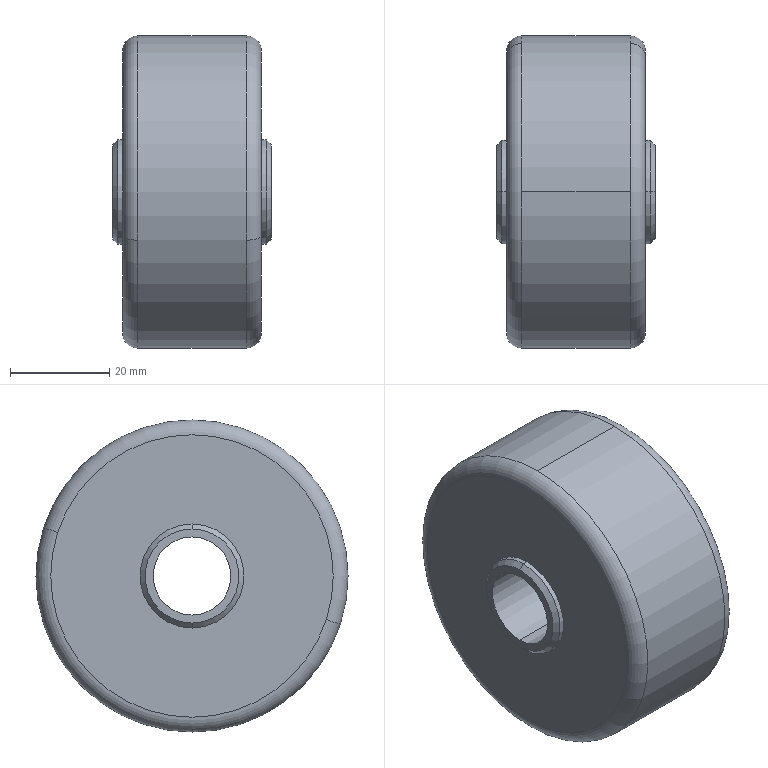Part | NX | features BREP 1 | 1 solid | 20 faces | box 32 x 63 x 63 mm | volume 81622 mm3 | cylinder 8 | cone 4 | plane 4 | torus 4 | commonest cylinder face diameters 21 x4 15.75 x2 63 x2
STEP:
#1=CARTESIAN_POINT('',(-16.,0.,-9.5));
#2=VERTEX_POINT('',#1);
#3=CARTESIAN_POINT('',(-16.,0.,9.5));
#4=VERTEX_POINT('',#3);
#5=CARTESIAN_POINT('',(-16.,0.,0.));
#6=DIRECTION('',(-1.,0.,0.));
#7=DIRECTION('',(0.,0.,-1.));
#8=AXIS2_PLACEMENT_3D('',#5,#6,#7);
#9=CIRCLE('',#8,9.5);
#10=EDGE_CURVE('',#2,#4,#9,.T.);
#11=ORIENTED_EDGE('',*,*,#10,.F.);
#12=CARTESIAN_POINT('',(-15.,0.,-10.5));
#13=VERTEX_POINT('',#12);
#14=CARTESIAN_POINT('',(-15.,0.,-10.5));
#15=DIRECTION('',(-0.7071,0.,0.7071));
#16=VECTOR('',#15,1000.);
#17=LINE('',#14,#16);
#18=EDGE_CURVE('',#2,#13,#17,.F.);
#19=ORIENTED_EDGE('',*,*,#18,.T.);
#20=CARTESIAN_POINT('',(-15.,0.,10.5));
#21=VERTEX_POINT('',#20);
#22=CARTESIAN_POINT('',(-15.,0.,0.));
#23=DIRECTION('',(-1.,0.,0.));
#24=DIRECTION('',(0.,0.,-1.));
#25=AXIS2_PLACEMENT_3D('',#22,#23,#24);
#26=CIRCLE('',#25,10.5);
#27=EDGE_CURVE('',#13,#21,#26,.T.);
#28=ORIENTED_EDGE('',*,*,#27,.T.);
#29=CARTESIAN_POINT('',(-15.,0.,10.5));
#30=DIRECTION('',(-0.7071,0.,-0.7071));
#31=VECTOR('',#30,1000.);
#32=LINE('',#29,#31);
#33=EDGE_CURVE('',#4,#21,#32,.F.);
#34=ORIENTED_EDGE('',*,*,#33,.F.);
#35=EDGE_LOOP('',(#11,#19,#28,#34));
#36=FACE_BOUND('',#35,.T.);
#37=CARTESIAN_POINT('',(-15.5,0.,0.));
#38=DIRECTION('',(1.,0.,0.));
#39=DIRECTION('',(0.,0.,1.));
#40=AXIS2_PLACEMENT_3D('',#37,#38,#39);
#41=CONICAL_SURFACE('',#40,10.,0.7854);
#42=ADVANCED_FACE('',(#36),#41,.T.);
#43=CARTESIAN_POINT('',(-15.,0.,0.));
#44=DIRECTION('',(-1.,0.,0.));
#45=DIRECTION('',(0.,0.,1.));
#46=AXIS2_PLACEMENT_3D('',#43,#44,#45);
#47=CIRCLE('',#46,10.5);
#48=EDGE_CURVE('',#21,#13,#47,.T.);
#49=ORIENTED_EDGE('',*,*,#48,.T.);
#50=ORIENTED_EDGE('',*,*,#18,.F.);
#51=CARTESIAN_POINT('',(-16.,0.,0.));
#52=DIRECTION('',(-1.,0.,0.));
#53=DIRECTION('',(0.,0.,1.));
#54=AXIS2_PLACEMENT_3D('',#51,#52,#53);
#55=CIRCLE('',#54,9.5);
#56=EDGE_CURVE('',#4,#2,#55,.T.);
#57=ORIENTED_EDGE('',*,*,#56,.F.);
#58=ORIENTED_EDGE('',*,*,#33,.T.);
#59=EDGE_LOOP('',(#49,#50,#57,#58));
#60=FACE_BOUND('',#59,.T.);
#61=CARTESIAN_POINT('',(-15.5,0.,0.));
#62=DIRECTION('',(1.,0.,0.));
#63=DIRECTION('',(0.,0.,-1.));
#64=AXIS2_PLACEMENT_3D('',#61,#62,#63);
#65=CONICAL_SURFACE('',#64,10.,0.7854);
#66=ADVANCED_FACE('',(#60),#65,.T.);
#67=ORIENTED_EDGE('',*,*,#56,.T.);
#68=ORIENTED_EDGE('',*,*,#10,.T.);
#69=EDGE_LOOP('',(#67,#68));
#70=FACE_BOUND('',#69,.T.);
#71=CARTESIAN_POINT('',(-16.,0.,7.875));
#72=VERTEX_POINT('',#71);
#73=CARTESIAN_POINT('',(-16.,0.,-7.875));
#74=VERTEX_POINT('',#73);
#75=CARTESIAN_POINT('',(-16.,0.,0.));
#76=DIRECTION('',(1.,0.,0.));
#77=DIRECTION('',(0.,0.,1.));
#78=AXIS2_PLACEMENT_3D('',#75,#76,#77);
#79=CIRCLE('',#78,7.875);
#80=EDGE_CURVE('',#72,#74,#79,.T.);
#81=ORIENTED_EDGE('',*,*,#80,.T.);
#82=CARTESIAN_POINT('',(-16.,0.,0.));
#83=DIRECTION('',(1.,0.,0.));
#84=DIRECTION('',(0.,0.,-1.));
#85=AXIS2_PLACEMENT_3D('',#82,#83,#84);
#86=CIRCLE('',#85,7.875);
#87=EDGE_CURVE('',#74,#72,#86,.T.);
#88=ORIENTED_EDGE('',*,*,#87,.T.);
#89=EDGE_LOOP('',(#81,#88));
#90=FACE_BOUND('',#89,.T.);
#91=CARTESIAN_POINT('',(-16.,9.5,0.));
#92=DIRECTION('',(-1.,0.,0.));
#93=DIRECTION('',(0.,0.,1.));
#94=AXIS2_PLACEMENT_3D('',#91,#92,#93);
#95=PLANE('',#94);
#96=ADVANCED_FACE('',(#70,#90),#95,.T.);
#97=ORIENTED_EDGE('',*,*,#87,.F.);
#98=CARTESIAN_POINT('',(16.,0.,-7.875));
#99=VERTEX_POINT('',#98);
#100=CARTESIAN_POINT('',(16.,0.,-7.875));
#101=DIRECTION('',(-1.,0.,0.));
#102=VECTOR('',#101,1000.);
#103=LINE('',#100,#102);
#104=EDGE_CURVE('',#74,#99,#103,.F.);
#105=ORIENTED_EDGE('',*,*,#104,.T.);
#106=CARTESIAN_POINT('',(16.,0.,7.875));
#107=VERTEX_POINT('',#106);
#108=CARTESIAN_POINT('',(16.,0.,0.));
#109=DIRECTION('',(-1.,0.,0.));
#110=DIRECTION('',(0.,0.,1.));
#111=AXIS2_PLACEMENT_3D('',#108,#109,#110);
#112=CIRCLE('',#111,7.875);
#113=EDGE_CURVE('',#107,#99,#112,.T.);
#114=ORIENTED_EDGE('',*,*,#113,.F.);
#115=CARTESIAN_POINT('',(16.,0.,7.875));
#116=DIRECTION('',(-1.,0.,0.));
#117=VECTOR('',#116,1000.);
#118=LINE('',#115,#117);
#119=EDGE_CURVE('',#72,#107,#118,.F.);
#120=ORIENTED_EDGE('',*,*,#119,.F.);
#121=EDGE_LOOP('',(#97,#105,#114,#120));
#122=FACE_BOUND('',#121,.T.);
#123=CARTESIAN_POINT('',(50.,0.,0.));
#124=DIRECTION('',(1.,0.,0.));
#125=DIRECTION('',(0.,0.,-1.));
#126=AXIS2_PLACEMENT_3D('',#123,#124,#125);
#127=CYLINDRICAL_SURFACE('',#126,7.875);
#128=ADVANCED_FACE('',(#122),#127,.F.);
#129=CARTESIAN_POINT('',(16.,0.,0.));
#130=DIRECTION('',(-1.,0.,0.));
#131=DIRECTION('',(0.,0.,-1.));
#132=AXIS2_PLACEMENT_3D('',#129,#130,#131);
#133=CIRCLE('',#132,7.875);
#134=EDGE_CURVE('',#99,#107,#133,.T.);
#135=ORIENTED_EDGE('',*,*,#134,.F.);
#136=ORIENTED_EDGE('',*,*,#104,.F.);
#137=ORIENTED_EDGE('',*,*,#80,.F.);
#138=ORIENTED_EDGE('',*,*,#119,.T.);
#139=EDGE_LOOP('',(#135,#136,#137,#138));
#140=FACE_BOUND('',#139,.T.);
#141=CARTESIAN_POINT('',(50.,0.,0.));
#142=DIRECTION('',(1.,0.,0.));
#143=DIRECTION('',(0.,0.,1.));
#144=AXIS2_PLACEMENT_3D('',#141,#142,#143);
#145=CYLINDRICAL_SURFACE('',#144,7.875);
#146=ADVANCED_FACE('',(#140),#145,.F.);
#147=CARTESIAN_POINT('',(16.,0.,9.5));
#148=VERTEX_POINT('',#147);
#149=CARTESIAN_POINT('',(16.,0.,-9.5));
#150=VERTEX_POINT('',#149);
#151=CARTESIAN_POINT('',(16.,0.,0.));
#152=DIRECTION('',(1.,0.,0.));
#153=DIRECTION('',(0.,0.,1.));
#154=AXIS2_PLACEMENT_3D('',#151,#152,#153);
#155=CIRCLE('',#154,9.5);
#156=EDGE_CURVE('',#148,#150,#155,.T.);
#157=ORIENTED_EDGE('',*,*,#156,.T.);
#158=CARTESIAN_POINT('',(16.,0.,0.));
#159=DIRECTION('',(1.,0.,0.));
#160=DIRECTION('',(0.,0.,-1.));
#161=AXIS2_PLACEMENT_3D('',#158,#159,#160);
#162=CIRCLE('',#161,9.5);
#163=EDGE_CURVE('',#150,#148,#162,.T.);
#164=ORIENTED_EDGE('',*,*,#163,.T.);
#165=EDGE_LOOP('',(#157,#164));
#166=FACE_BOUND('',#165,.T.);
#167=ORIENTED_EDGE('',*,*,#113,.T.);
#168=ORIENTED_EDGE('',*,*,#134,.T.);
#169=EDGE_LOOP('',(#167,#168));
#170=FACE_BOUND('',#169,.T.);
#171=CARTESIAN_POINT('',(16.,7.875,0.));
#172=DIRECTION('',(1.,0.,0.));
#173=DIRECTION('',(0.,1.,0.));
#174=AXIS2_PLACEMENT_3D('',#171,#172,#173);
#175=PLANE('',#174);
#176=ADVANCED_FACE('',(#166,#170),#175,.T.);
#177=CARTESIAN_POINT('',(15.,0.,-10.5));
#178=VERTEX_POINT('',#177);
#179=CARTESIAN_POINT('',(15.,0.,10.5));
#180=VERTEX_POINT('',#179);
#181=CARTESIAN_POINT('',(15.,0.,0.));
#182=DIRECTION('',(1.,0.,0.));
#183=DIRECTION('',(0.,0.,-1.));
#184=AXIS2_PLACEMENT_3D('',#181,#182,#183);
#185=CIRCLE('',#184,10.5);
#186=EDGE_CURVE('',#178,#180,#185,.T.);
#187=ORIENTED_EDGE('',*,*,#186,.T.);
#188=CARTESIAN_POINT('',(15.,0.,10.5));
#189=DIRECTION('',(0.7071,0.,-0.7071));
#190=VECTOR('',#189,1000.);
#191=LINE('',#188,#190);
#192=EDGE_CURVE('',#180,#148,#191,.T.);
#193=ORIENTED_EDGE('',*,*,#192,.T.);
#194=ORIENTED_EDGE('',*,*,#163,.F.);
#195=CARTESIAN_POINT('',(15.,0.,-10.5));
#196=DIRECTION('',(0.7071,0.,0.7071));
#197=VECTOR('',#196,1000.);
#198=LINE('',#195,#197);
#199=EDGE_CURVE('',#178,#150,#198,.T.);
#200=ORIENTED_EDGE('',*,*,#199,.F.);
#201=EDGE_LOOP('',(#187,#193,#194,#200));
#202=FACE_BOUND('',#201,.T.);
#203=CARTESIAN_POINT('',(15.5,0.,0.));
#204=DIRECTION('',(-1.,0.,0.));
#205=DIRECTION('',(0.,0.,1.));
#206=AXIS2_PLACEMENT_3D('',#203,#204,#205);
#207=CONICAL_SURFACE('',#206,10.,0.7854);
#208=ADVANCED_FACE('',(#202),#207,.T.);
#209=ORIENTED_EDGE('',*,*,#156,.F.);
#210=ORIENTED_EDGE('',*,*,#192,.F.);
#211=CARTESIAN_POINT('',(15.,0.,0.));
#212=DIRECTION('',(1.,0.,0.));
#213=DIRECTION('',(0.,0.,1.));
#214=AXIS2_PLACEMENT_3D('',#211,#212,#213);
#215=CIRCLE('',#214,10.5);
#216=EDGE_CURVE('',#180,#178,#215,.T.);
#217=ORIENTED_EDGE('',*,*,#216,.T.);
#218=ORIENTED_EDGE('',*,*,#199,.T.);
#219=EDGE_LOOP('',(#209,#210,#217,#218));
#220=FACE_BOUND('',#219,.T.);
#221=CARTESIAN_POINT('',(15.5,0.,0.));
#222=DIRECTION('',(-1.,0.,0.));
#223=DIRECTION('',(0.,0.,-1.));
#224=AXIS2_PLACEMENT_3D('',#221,#222,#223);
#225=CONICAL_SURFACE('',#224,10.,0.7854);
#226=ADVANCED_FACE('',(#220),#225,.T.);
#227=CARTESIAN_POINT('',(14.,0.,-10.5));
#228=VERTEX_POINT('',#227);
#229=CARTESIAN_POINT('',(14.,0.,10.5));
#230=VERTEX_POINT('',#229);
#231=CARTESIAN_POINT('',(14.,0.,0.));
#232=DIRECTION('',(-1.,0.,0.));
#233=DIRECTION('',(0.,0.,-1.));
#234=AXIS2_PLACEMENT_3D('',#231,#232,#233);
#235=CIRCLE('',#234,10.5);
#236=EDGE_CURVE('',#228,#230,#235,.T.);
#237=ORIENTED_EDGE('',*,*,#236,.F.);
#238=CARTESIAN_POINT('',(15.,0.,-10.5));
#239=DIRECTION('',(-1.,0.,0.));
#240=VECTOR('',#239,1000.);
#241=LINE('',#238,#240);
#242=EDGE_CURVE('',#228,#178,#241,.F.);
#243=ORIENTED_EDGE('',*,*,#242,.T.);
#244=ORIENTED_EDGE('',*,*,#216,.F.);
#245=CARTESIAN_POINT('',(15.,0.,10.5));
#246=DIRECTION('',(-1.,0.,0.));
#247=VECTOR('',#246,1000.);
#248=LINE('',#245,#247);
#249=EDGE_CURVE('',#230,#180,#248,.F.);
#250=ORIENTED_EDGE('',*,*,#249,.F.);
#251=EDGE_LOOP('',(#237,#243,#244,#250));
#252=FACE_BOUND('',#251,.T.);
#253=CARTESIAN_POINT('',(50.,0.,0.));
#254=DIRECTION('',(1.,0.,0.));
#255=DIRECTION('',(0.,0.,1.));
#256=AXIS2_PLACEMENT_3D('',#253,#254,#255);
#257=CYLINDRICAL_SURFACE('',#256,10.5);
#258=ADVANCED_FACE('',(#252),#257,.T.);
#259=ORIENTED_EDGE('',*,*,#186,.F.);
#260=ORIENTED_EDGE('',*,*,#242,.F.);
#261=CARTESIAN_POINT('',(14.,0.,0.));
#262=DIRECTION('',(-1.,0.,0.));
#263=DIRECTION('',(0.,0.,1.));
#264=AXIS2_PLACEMENT_3D('',#261,#262,#263);
#265=CIRCLE('',#264,10.5);
#266=EDGE_CURVE('',#230,#228,#265,.T.);
#267=ORIENTED_EDGE('',*,*,#266,.F.);
#268=ORIENTED_EDGE('',*,*,#249,.T.);
#269=EDGE_LOOP('',(#259,#260,#267,#268));
#270=FACE_BOUND('',#269,.T.);
#271=CARTESIAN_POINT('',(50.,0.,0.));
#272=DIRECTION('',(1.,0.,0.));
#273=DIRECTION('',(0.,0.,-1.));
#274=AXIS2_PLACEMENT_3D('',#271,#272,#273);
#275=CYLINDRICAL_SURFACE('',#274,10.5);
#276=ADVANCED_FACE('',(#270),#275,.T.);
#277=CARTESIAN_POINT('',(14.,27.105,8.807));
#278=VERTEX_POINT('',#277);
#279=CARTESIAN_POINT('',(14.,-27.105,-8.807));
#280=VERTEX_POINT('',#279);
#281=CARTESIAN_POINT('',(14.,0.,0.));
#282=DIRECTION('',(1.,0.,0.));
#283=DIRECTION('',(0.,0.9511,0.309));
#284=AXIS2_PLACEMENT_3D('',#281,#282,#283);
#285=CIRCLE('',#284,28.5);
#286=EDGE_CURVE('',#278,#280,#285,.T.);
#287=ORIENTED_EDGE('',*,*,#286,.T.);
#288=CARTESIAN_POINT('',(14.,0.,0.));
#289=DIRECTION('',(1.,0.,0.));
#290=DIRECTION('',(0.,-0.9511,-0.309));
#291=AXIS2_PLACEMENT_3D('',#288,#289,#290);
#292=CIRCLE('',#291,28.5);
#293=EDGE_CURVE('',#280,#278,#292,.T.);
#294=ORIENTED_EDGE('',*,*,#293,.T.);
#295=EDGE_LOOP('',(#287,#294));
#296=FACE_BOUND('',#295,.T.);
#297=ORIENTED_EDGE('',*,*,#266,.T.);
#298=ORIENTED_EDGE('',*,*,#236,.T.);
#299=EDGE_LOOP('',(#297,#298));
#300=FACE_BOUND('',#299,.T.);
#301=CARTESIAN_POINT('',(14.,10.5,0.));
#302=DIRECTION('',(1.,0.,0.));
#303=DIRECTION('',(0.,1.,0.));
#304=AXIS2_PLACEMENT_3D('',#301,#302,#303);
#305=PLANE('',#304);
#306=ADVANCED_FACE('',(#296,#300),#305,.T.);
#307=CARTESIAN_POINT('',(11.,-29.958,-9.734));
#308=VERTEX_POINT('',#307);
#309=CARTESIAN_POINT('',(11.,0.,-31.5));
#310=VERTEX_POINT('',#309);
#311=CARTESIAN_POINT('',(11.,0.,0.));
#312=DIRECTION('',(1.,0.,0.));
#313=DIRECTION('',(0.,-0.9511,-0.309));
#314=AXIS2_PLACEMENT_3D('',#311,#312,#313);
#315=CIRCLE('',#314,31.5);
#316=EDGE_CURVE('',#308,#310,#315,.T.);
#317=ORIENTED_EDGE('',*,*,#316,.T.);
#318=CARTESIAN_POINT('',(11.,29.958,9.734));
#319=VERTEX_POINT('',#318);
#320=CARTESIAN_POINT('',(11.,0.,0.));
#321=DIRECTION('',(1.,0.,0.));
#322=DIRECTION('',(0.,0.,-1.));
#323=AXIS2_PLACEMENT_3D('',#320,#321,#322);
#324=CIRCLE('',#323,31.5);
#325=EDGE_CURVE('',#310,#319,#324,.T.);
#326=ORIENTED_EDGE('',*,*,#325,.T.);
#327=CARTESIAN_POINT('',(11.,27.105,8.807));
#328=DIRECTION('',(0.,0.309,-0.9511));
#329=DIRECTION('',(0.,0.9511,0.309));
#330=AXIS2_PLACEMENT_3D('',#327,#328,#329);
#331=CIRCLE('',#330,3.);
#332=EDGE_CURVE('',#319,#278,#331,.T.);
#333=ORIENTED_EDGE('',*,*,#332,.T.);
#334=ORIENTED_EDGE('',*,*,#293,.F.);
#335=CARTESIAN_POINT('',(11.,-27.105,-8.807));
#336=DIRECTION('',(0.,-0.309,0.9511));
#337=DIRECTION('',(0.,-0.9511,-0.309));
#338=AXIS2_PLACEMENT_3D('',#335,#336,#337);
#339=CIRCLE('',#338,3.);
#340=EDGE_CURVE('',#308,#280,#339,.T.);
#341=ORIENTED_EDGE('',*,*,#340,.F.);
#342=EDGE_LOOP('',(#317,#326,#333,#334,#341));
#343=FACE_BOUND('',#342,.T.);
#344=CARTESIAN_POINT('',(11.,0.,0.));
#345=DIRECTION('',(1.,0.,0.));
#346=DIRECTION('',(0.,-0.9511,-0.309));
#347=AXIS2_PLACEMENT_3D('',#344,#345,#346);
#348=TOROIDAL_SURFACE('',#347,28.5,3.);
#349=ADVANCED_FACE('',(#343),#348,.T.);
#350=ORIENTED_EDGE('',*,*,#286,.F.);
#351=ORIENTED_EDGE('',*,*,#332,.F.);
#352=CARTESIAN_POINT('',(11.,0.,31.5));
#353=VERTEX_POINT('',#352);
#354=CARTESIAN_POINT('',(11.,0.,0.));
#355=DIRECTION('',(1.,0.,0.));
#356=DIRECTION('',(0.,0.9511,0.309));
#357=AXIS2_PLACEMENT_3D('',#354,#355,#356);
#358=CIRCLE('',#357,31.5);
#359=EDGE_CURVE('',#319,#353,#358,.T.);
#360=ORIENTED_EDGE('',*,*,#359,.T.);
#361=CARTESIAN_POINT('',(11.,0.,0.));
#362=DIRECTION('',(1.,0.,0.));
#363=DIRECTION('',(0.,0.,1.));
#364=AXIS2_PLACEMENT_3D('',#361,#362,#363);
#365=CIRCLE('',#364,31.5);
#366=EDGE_CURVE('',#353,#308,#365,.T.);
#367=ORIENTED_EDGE('',*,*,#366,.T.);
#368=ORIENTED_EDGE('',*,*,#340,.T.);
#369=EDGE_LOOP('',(#350,#351,#360,#367,#368));
#370=FACE_BOUND('',#369,.T.);
#371=CARTESIAN_POINT('',(11.,0.,0.));
#372=DIRECTION('',(1.,0.,0.));
#373=DIRECTION('',(0.,0.9511,0.309));
#374=AXIS2_PLACEMENT_3D('',#371,#372,#373);
#375=TOROIDAL_SURFACE('',#374,28.5,3.);
#376=ADVANCED_FACE('',(#370),#375,.T.);
#377=CARTESIAN_POINT('',(-11.,-29.958,-9.734));
#378=VERTEX_POINT('',#377);
#379=CARTESIAN_POINT('',(-11.,0.,31.5));
#380=VERTEX_POINT('',#379);
#381=CARTESIAN_POINT('',(-11.,0.,0.));
#382=DIRECTION('',(-1.,0.,0.));
#383=DIRECTION('',(0.,-0.9511,-0.309));
#384=AXIS2_PLACEMENT_3D('',#381,#382,#383);
#385=CIRCLE('',#384,31.5);
#386=EDGE_CURVE('',#378,#380,#385,.T.);
#387=ORIENTED_EDGE('',*,*,#386,.F.);
#388=CARTESIAN_POINT('',(-11.,0.,-31.5));
#389=VERTEX_POINT('',#388);
#390=CARTESIAN_POINT('',(-11.,0.,0.));
#391=DIRECTION('',(-1.,0.,0.));
#392=DIRECTION('',(0.,0.,-1.));
#393=AXIS2_PLACEMENT_3D('',#390,#391,#392);
#394=CIRCLE('',#393,31.5);
#395=EDGE_CURVE('',#389,#378,#394,.T.);
#396=ORIENTED_EDGE('',*,*,#395,.F.);
#397=CARTESIAN_POINT('',(11.,0.,-31.5));
#398=DIRECTION('',(-1.,0.,0.));
#399=VECTOR('',#398,1000.);
#400=LINE('',#397,#399);
#401=EDGE_CURVE('',#389,#310,#400,.F.);
#402=ORIENTED_EDGE('',*,*,#401,.T.);
#403=ORIENTED_EDGE('',*,*,#316,.F.);
#404=ORIENTED_EDGE('',*,*,#366,.F.);
#405=CARTESIAN_POINT('',(11.,0.,31.5));
#406=DIRECTION('',(-1.,0.,0.));
#407=VECTOR('',#406,1000.);
#408=LINE('',#405,#407);
#409=EDGE_CURVE('',#380,#353,#408,.F.);
#410=ORIENTED_EDGE('',*,*,#409,.F.);
#411=EDGE_LOOP('',(#387,#396,#402,#403,#404,#410));
#412=FACE_BOUND('',#411,.T.);
#413=CARTESIAN_POINT('',(50.,0.,0.));
#414=DIRECTION('',(1.,0.,0.));
#415=DIRECTION('',(0.,0.,1.));
#416=AXIS2_PLACEMENT_3D('',#413,#414,#415);
#417=CYLINDRICAL_SURFACE('',#416,31.5);
#418=ADVANCED_FACE('',(#412),#417,.T.);
#419=ORIENTED_EDGE('',*,*,#359,.F.);
#420=ORIENTED_EDGE('',*,*,#325,.F.);
#421=ORIENTED_EDGE('',*,*,#401,.F.);
#422=CARTESIAN_POINT('',(-11.,29.958,9.734));
#423=VERTEX_POINT('',#422);
#424=CARTESIAN_POINT('',(-11.,0.,0.));
#425=DIRECTION('',(-1.,0.,0.));
#426=DIRECTION('',(0.,0.9511,0.309));
#427=AXIS2_PLACEMENT_3D('',#424,#425,#426);
#428=CIRCLE('',#427,31.5);
#429=EDGE_CURVE('',#423,#389,#428,.T.);
#430=ORIENTED_EDGE('',*,*,#429,.F.);
#431=CARTESIAN_POINT('',(-11.,0.,0.));
#432=DIRECTION('',(-1.,0.,0.));
#433=DIRECTION('',(0.,0.,1.));
#434=AXIS2_PLACEMENT_3D('',#431,#432,#433);
#435=CIRCLE('',#434,31.5);
#436=EDGE_CURVE('',#380,#423,#435,.T.);
#437=ORIENTED_EDGE('',*,*,#436,.F.);
#438=ORIENTED_EDGE('',*,*,#409,.T.);
#439=EDGE_LOOP('',(#419,#420,#421,#430,#437,#438));
#440=FACE_BOUND('',#439,.T.);
#441=CARTESIAN_POINT('',(50.,0.,0.));
#442=DIRECTION('',(1.,0.,0.));
#443=DIRECTION('',(0.,0.,-1.));
#444=AXIS2_PLACEMENT_3D('',#441,#442,#443);
#445=CYLINDRICAL_SURFACE('',#444,31.5);
#446=ADVANCED_FACE('',(#440),#445,.T.);
#447=ORIENTED_EDGE('',*,*,#386,.T.);
#448=ORIENTED_EDGE('',*,*,#436,.T.);
#449=CARTESIAN_POINT('',(-14.,27.105,8.807));
#450=VERTEX_POINT('',#449);
#451=CARTESIAN_POINT('',(-11.,27.105,8.807));
#452=DIRECTION('',(0.,0.309,-0.9511));
#453=DIRECTION('',(-1.,0.,0.));
#454=AXIS2_PLACEMENT_3D('',#451,#452,#453);
#455=CIRCLE('',#454,3.);
#456=EDGE_CURVE('',#450,#423,#455,.T.);
#457=ORIENTED_EDGE('',*,*,#456,.F.);
#458=CARTESIAN_POINT('',(-14.,-27.105,-8.807));
#459=VERTEX_POINT('',#458);
#460=CARTESIAN_POINT('',(-14.,0.,0.));
#461=DIRECTION('',(-1.,0.,0.));
#462=DIRECTION('',(0.,-0.9511,-0.309));
#463=AXIS2_PLACEMENT_3D('',#460,#461,#462);
#464=CIRCLE('',#463,28.5);
#465=EDGE_CURVE('',#459,#450,#464,.T.);
#466=ORIENTED_EDGE('',*,*,#465,.F.);
#467=CARTESIAN_POINT('',(-11.,-27.105,-8.807));
#468=DIRECTION('',(0.,-0.309,0.9511));
#469=DIRECTION('',(-1.,0.,0.));
#470=AXIS2_PLACEMENT_3D('',#467,#468,#469);
#471=CIRCLE('',#470,3.);
#472=EDGE_CURVE('',#459,#378,#471,.T.);
#473=ORIENTED_EDGE('',*,*,#472,.T.);
#474=EDGE_LOOP('',(#447,#448,#457,#466,#473));
#475=FACE_BOUND('',#474,.T.);
#476=CARTESIAN_POINT('',(-11.,0.,0.));
#477=DIRECTION('',(1.,0.,0.));
#478=DIRECTION('',(0.,0.9511,0.309));
#479=AXIS2_PLACEMENT_3D('',#476,#477,#478);
#480=TOROIDAL_SURFACE('',#479,28.5,3.);
#481=ADVANCED_FACE('',(#475),#480,.T.);
#482=CARTESIAN_POINT('',(-14.,0.,0.));
#483=DIRECTION('',(-1.,0.,0.));
#484=DIRECTION('',(0.,0.,-1.));
#485=AXIS2_PLACEMENT_3D('',#482,#483,#484);
#486=CIRCLE('',#485,28.5);
#487=EDGE_CURVE('',#450,#459,#486,.T.);
#488=ORIENTED_EDGE('',*,*,#487,.F.);
#489=ORIENTED_EDGE('',*,*,#456,.T.);
#490=ORIENTED_EDGE('',*,*,#429,.T.);
#491=ORIENTED_EDGE('',*,*,#395,.T.);
#492=ORIENTED_EDGE('',*,*,#472,.F.);
#493=EDGE_LOOP('',(#488,#489,#490,#491,#492));
#494=FACE_BOUND('',#493,.T.);
#495=CARTESIAN_POINT('',(-11.,0.,0.));
#496=DIRECTION('',(1.,0.,0.));
#497=DIRECTION('',(0.,-0.9511,-0.309));
#498=AXIS2_PLACEMENT_3D('',#495,#496,#497);
#499=TOROIDAL_SURFACE('',#498,28.5,3.);
#500=ADVANCED_FACE('',(#494),#499,.T.);
#501=ORIENTED_EDGE('',*,*,#465,.T.);
#502=ORIENTED_EDGE('',*,*,#487,.T.);
#503=EDGE_LOOP('',(#501,#502));
#504=FACE_BOUND('',#503,.T.);
#505=CARTESIAN_POINT('',(-14.,0.,10.5));
#506=VERTEX_POINT('',#505);
#507=CARTESIAN_POINT('',(-14.,0.,-10.5));
#508=VERTEX_POINT('',#507);
#509=CARTESIAN_POINT('',(-14.,0.,0.));
#510=DIRECTION('',(1.,0.,0.));
#511=DIRECTION('',(0.,0.,1.));
#512=AXIS2_PLACEMENT_3D('',#509,#510,#511);
#513=CIRCLE('',#512,10.5);
#514=EDGE_CURVE('',#506,#508,#513,.T.);
#515=ORIENTED_EDGE('',*,*,#514,.T.);
#516=CARTESIAN_POINT('',(-14.,0.,0.));
#517=DIRECTION('',(1.,0.,0.));
#518=DIRECTION('',(0.,0.,-1.));
#519=AXIS2_PLACEMENT_3D('',#516,#517,#518);
#520=CIRCLE('',#519,10.5);
#521=EDGE_CURVE('',#508,#506,#520,.T.);
#522=ORIENTED_EDGE('',*,*,#521,.T.);
#523=EDGE_LOOP('',(#515,#522));
#524=FACE_BOUND('',#523,.T.);
#525=CARTESIAN_POINT('',(-14.,28.5,0.));
#526=DIRECTION('',(-1.,0.,0.));
#527=DIRECTION('',(0.,0.,1.));
#528=AXIS2_PLACEMENT_3D('',#525,#526,#527);
#529=PLANE('',#528);
#530=ADVANCED_FACE('',(#504,#524),#529,.T.);
#531=ORIENTED_EDGE('',*,*,#521,.F.);
#532=CARTESIAN_POINT('',(-14.,0.,-10.5));
#533=DIRECTION('',(-1.,0.,0.));
#534=VECTOR('',#533,1000.);
#535=LINE('',#532,#534);
#536=EDGE_CURVE('',#13,#508,#535,.F.);
#537=ORIENTED_EDGE('',*,*,#536,.F.);
#538=ORIENTED_EDGE('',*,*,#48,.F.);
#539=CARTESIAN_POINT('',(-14.,0.,10.5));
#540=DIRECTION('',(-1.,0.,0.));
#541=VECTOR('',#540,1000.);
#542=LINE('',#539,#541);
#543=EDGE_CURVE('',#21,#506,#542,.F.);
#544=ORIENTED_EDGE('',*,*,#543,.T.);
#545=EDGE_LOOP('',(#531,#537,#538,#544));
#546=FACE_BOUND('',#545,.T.);
#547=CARTESIAN_POINT('',(50.,0.,0.));
#548=DIRECTION('',(1.,0.,0.));
#549=DIRECTION('',(0.,0.,-1.));
#550=AXIS2_PLACEMENT_3D('',#547,#548,#549);
#551=CYLINDRICAL_SURFACE('',#550,10.5);
#552=ADVANCED_FACE('',(#546),#551,.T.);
#553=ORIENTED_EDGE('',*,*,#27,.F.);
#554=ORIENTED_EDGE('',*,*,#536,.T.);
#555=ORIENTED_EDGE('',*,*,#514,.F.);
#556=ORIENTED_EDGE('',*,*,#543,.F.);
#557=EDGE_LOOP('',(#553,#554,#555,#556));
#558=FACE_BOUND('',#557,.T.);
#559=CARTESIAN_POINT('',(50.,0.,0.));
#560=DIRECTION('',(1.,0.,0.));
#561=DIRECTION('',(0.,0.,1.));
#562=AXIS2_PLACEMENT_3D('',#559,#560,#561);
#563=CYLINDRICAL_SURFACE('',#562,10.5);
#564=ADVANCED_FACE('',(#558),#563,.T.);
#565=CLOSED_SHELL('',(#42,#66,#96,#128,#146,#176,#208,#226,#258,#276,#306,#349,#376,#418,#446,#481,#500,#530,#552,#564));
#566=MANIFOLD_SOLID_BREP('',#565);
#567=(LENGTH_UNIT()NAMED_UNIT(*)SI_UNIT(.MILLI.,.METRE.));
#568=UNCERTAINTY_MEASURE_WITH_UNIT(LENGTH_MEASURE(0.00001),#567,'','');
#569=(NAMED_UNIT(*)PLANE_ANGLE_UNIT()SI_UNIT($,.RADIAN.));
#570=(NAMED_UNIT(*)SI_UNIT($,.STERADIAN.)SOLID_ANGLE_UNIT());
#571=(GEOMETRIC_REPRESENTATION_CONTEXT(3)GLOBAL_UNCERTAINTY_ASSIGNED_CONTEXT((#568))GLOBAL_UNIT_ASSIGNED_CONTEXT((#567,#569,#570))REPRESENTATION_CONTEXT('',''));
#572=ADVANCED_BREP_SHAPE_REPRESENTATION('',(#566),#571);